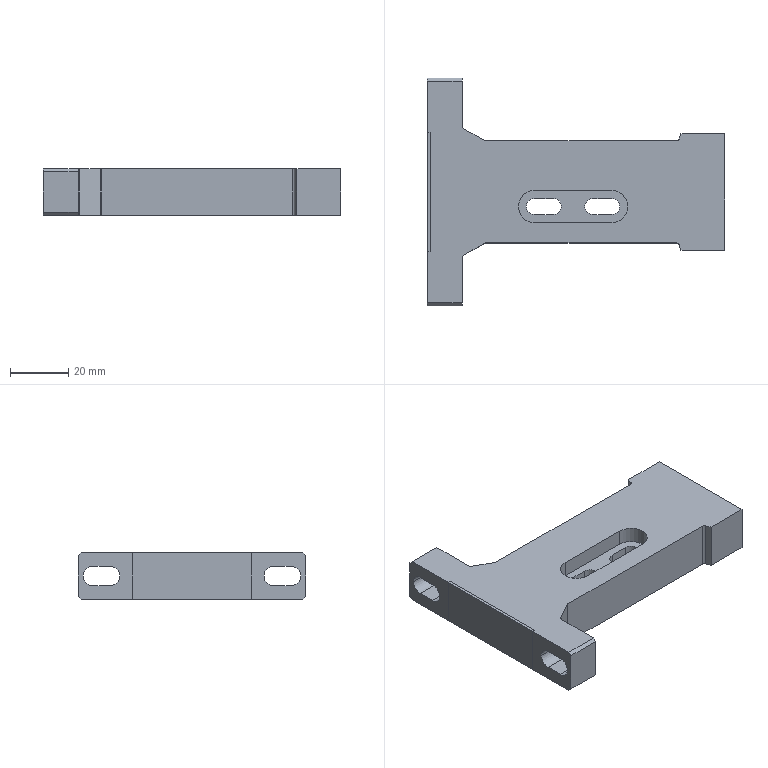Part | 2 solids | 79 faces | box 102 x 78 x 16 mm | volume 56779 mm3 | plane 45 | cylinder 26 | cone 8 | commonest cylinder face diameters 2 x6 6.6 x6 4 x4 5 x4 5.5 x4 11 x2